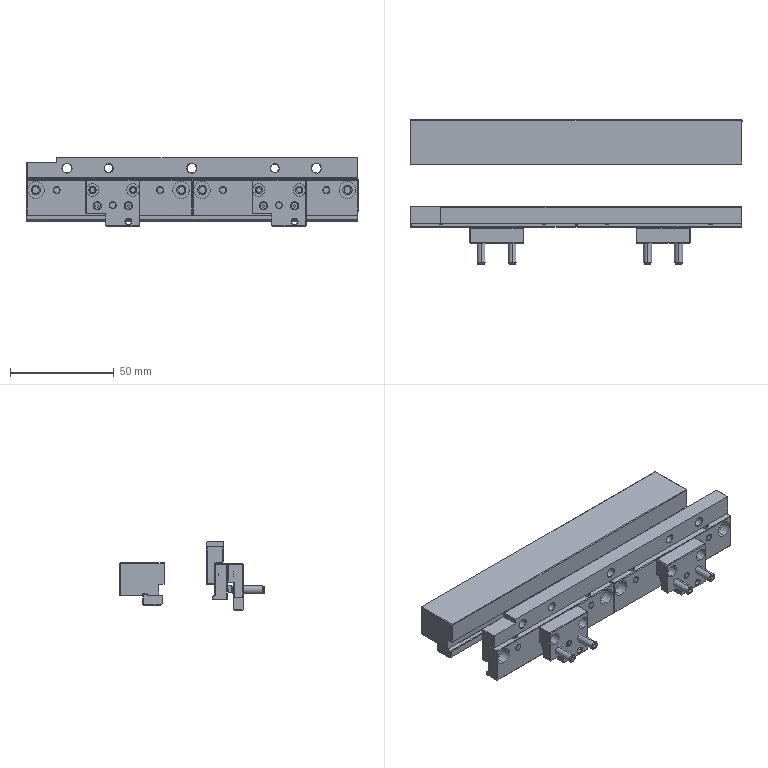Part | NX | 19 solids | 597 faces | box 159.75 x 69.305 x 32.9 mm | volume 98558 mm3 | plane 289 | cylinder 188 | cone 114 | sphere 6 | commonest cylinder face diameters 2.5 x36 3 x34 3.3 x28 4 x16 3.5 x14 4.5 x14